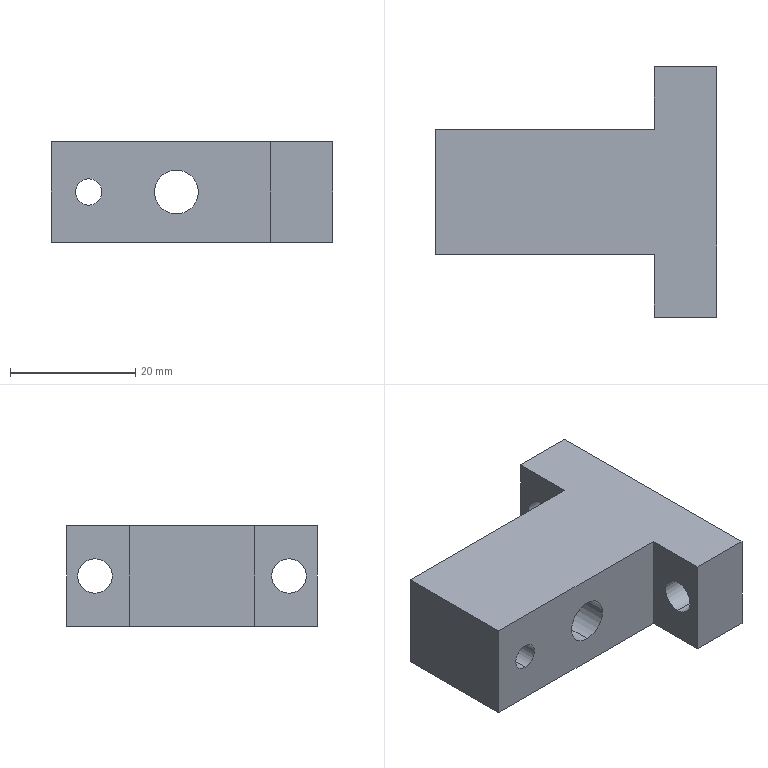Part | STEP file | 11-FG-E01311 | 1 solid | 24 faces | box 45 x 40 x 16 mm | volume 15803 mm3 | cylinder 12 | plane 12 | commonest cylinder face diameters 5 x4 5.5 x4 4.2 x2 7 x2
STEP:
#1=CARTESIAN_POINT('',(15.5,-5.5,10.5));
#2=VERTEX_POINT('',#1);
#3=CARTESIAN_POINT('',(15.5,-5.5,5.5));
#4=VERTEX_POINT('',#3);
#5=CARTESIAN_POINT('',(15.5,-5.5,8.));
#6=DIRECTION('',(1.,0.,0.));
#7=DIRECTION('',(0.,0.,-1.));
#8=AXIS2_PLACEMENT_3D('',#5,#6,#7);
#9=CIRCLE('',#8,2.5);
#10=EDGE_CURVE('',#2,#4,#9,.T.);
#11=ORIENTED_EDGE('',*,*,#10,.F.);
#12=CARTESIAN_POINT('',(22.5,-5.5,10.5));
#13=VERTEX_POINT('',#12);
#14=CARTESIAN_POINT('',(15.5,-5.5,10.5));
#15=DIRECTION('',(1.,0.,0.));
#16=VECTOR('',#15,1000.);
#17=LINE('',#14,#16);
#18=EDGE_CURVE('',#2,#13,#17,.T.);
#19=ORIENTED_EDGE('',*,*,#18,.T.);
#20=CARTESIAN_POINT('',(22.5,-5.5,5.5));
#21=VERTEX_POINT('',#20);
#22=CARTESIAN_POINT('',(22.5,-5.5,8.));
#23=DIRECTION('',(1.,0.,0.));
#24=DIRECTION('',(0.,0.,-1.));
#25=AXIS2_PLACEMENT_3D('',#22,#23,#24);
#26=CIRCLE('',#25,2.5);
#27=EDGE_CURVE('',#13,#21,#26,.T.);
#28=ORIENTED_EDGE('',*,*,#27,.T.);
#29=CARTESIAN_POINT('',(15.5,-5.5,5.5));
#30=DIRECTION('',(1.,0.,0.));
#31=VECTOR('',#30,1000.);
#32=LINE('',#29,#31);
#33=EDGE_CURVE('',#4,#21,#32,.T.);
#34=ORIENTED_EDGE('',*,*,#33,.F.);
#35=EDGE_LOOP('',(#11,#19,#28,#34));
#36=FACE_OUTER_BOUND('',#35,.T.);
#37=CARTESIAN_POINT('',(15.5,-5.5,8.));
#38=DIRECTION('',(1.,0.,0.));
#39=DIRECTION('',(0.,0.,-1.));
#40=AXIS2_PLACEMENT_3D('',#37,#38,#39);
#41=CYLINDRICAL_SURFACE('',#40,2.5);
#42=ADVANCED_FACE('',(#36),#41,.F.);
#43=CARTESIAN_POINT('',(15.5,5.5,10.5));
#44=VERTEX_POINT('',#43);
#45=CARTESIAN_POINT('',(15.5,5.5,5.5));
#46=VERTEX_POINT('',#45);
#47=CARTESIAN_POINT('',(15.5,5.5,8.));
#48=DIRECTION('',(1.,0.,0.));
#49=DIRECTION('',(0.,0.,-1.));
#50=AXIS2_PLACEMENT_3D('',#47,#48,#49);
#51=CIRCLE('',#50,2.5);
#52=EDGE_CURVE('',#44,#46,#51,.T.);
#53=ORIENTED_EDGE('',*,*,#52,.F.);
#54=CARTESIAN_POINT('',(22.5,5.5,10.5));
#55=VERTEX_POINT('',#54);
#56=CARTESIAN_POINT('',(15.5,5.5,10.5));
#57=DIRECTION('',(1.,0.,0.));
#58=VECTOR('',#57,1000.);
#59=LINE('',#56,#58);
#60=EDGE_CURVE('',#44,#55,#59,.T.);
#61=ORIENTED_EDGE('',*,*,#60,.T.);
#62=CARTESIAN_POINT('',(22.5,5.5,5.5));
#63=VERTEX_POINT('',#62);
#64=CARTESIAN_POINT('',(22.5,5.5,8.));
#65=DIRECTION('',(1.,0.,0.));
#66=DIRECTION('',(0.,0.,-1.));
#67=AXIS2_PLACEMENT_3D('',#64,#65,#66);
#68=CIRCLE('',#67,2.5);
#69=EDGE_CURVE('',#55,#63,#68,.T.);
#70=ORIENTED_EDGE('',*,*,#69,.T.);
#71=CARTESIAN_POINT('',(15.5,5.5,5.5));
#72=DIRECTION('',(1.,0.,0.));
#73=VECTOR('',#72,1000.);
#74=LINE('',#71,#73);
#75=EDGE_CURVE('',#46,#63,#74,.T.);
#76=ORIENTED_EDGE('',*,*,#75,.F.);
#77=EDGE_LOOP('',(#53,#61,#70,#76));
#78=FACE_OUTER_BOUND('',#77,.T.);
#79=CARTESIAN_POINT('',(15.5,5.5,8.));
#80=DIRECTION('',(1.,0.,0.));
#81=DIRECTION('',(0.,0.,-1.));
#82=AXIS2_PLACEMENT_3D('',#79,#80,#81);
#83=CYLINDRICAL_SURFACE('',#82,2.5);
#84=ADVANCED_FACE('',(#78),#83,.F.);
#85=CARTESIAN_POINT('',(22.5,-15.5,5.25));
#86=VERTEX_POINT('',#85);
#87=CARTESIAN_POINT('',(22.5,-15.5,10.75));
#88=VERTEX_POINT('',#87);
#89=CARTESIAN_POINT('',(22.5,-15.5,8.));
#90=DIRECTION('',(-1.,0.,0.));
#91=DIRECTION('',(0.,0.,1.));
#92=AXIS2_PLACEMENT_3D('',#89,#90,#91);
#93=CIRCLE('',#92,2.75);
#94=EDGE_CURVE('',#86,#88,#93,.T.);
#95=ORIENTED_EDGE('',*,*,#94,.F.);
#96=CARTESIAN_POINT('',(12.5,-15.5,5.25));
#97=VERTEX_POINT('',#96);
#98=CARTESIAN_POINT('',(27.5,-15.5,5.25));
#99=DIRECTION('',(-1.,0.,0.));
#100=VECTOR('',#99,1000.);
#101=LINE('',#98,#100);
#102=EDGE_CURVE('',#86,#97,#101,.T.);
#103=ORIENTED_EDGE('',*,*,#102,.T.);
#104=CARTESIAN_POINT('',(12.5,-15.5,10.75));
#105=VERTEX_POINT('',#104);
#106=CARTESIAN_POINT('',(12.5,-15.5,8.));
#107=DIRECTION('',(-1.,0.,0.));
#108=DIRECTION('',(0.,0.,1.));
#109=AXIS2_PLACEMENT_3D('',#106,#107,#108);
#110=CIRCLE('',#109,2.75);
#111=EDGE_CURVE('',#97,#105,#110,.T.);
#112=ORIENTED_EDGE('',*,*,#111,.T.);
#113=CARTESIAN_POINT('',(27.5,-15.5,10.75));
#114=DIRECTION('',(-1.,0.,0.));
#115=VECTOR('',#114,1000.);
#116=LINE('',#113,#115);
#117=EDGE_CURVE('',#88,#105,#116,.T.);
#118=ORIENTED_EDGE('',*,*,#117,.F.);
#119=EDGE_LOOP('',(#95,#103,#112,#118));
#120=FACE_OUTER_BOUND('',#119,.T.);
#121=CARTESIAN_POINT('',(27.5,-15.5,8.));
#122=DIRECTION('',(-1.,0.,0.));
#123=DIRECTION('',(0.,0.,1.));
#124=AXIS2_PLACEMENT_3D('',#121,#122,#123);
#125=CYLINDRICAL_SURFACE('',#124,2.75);
#126=ADVANCED_FACE('',(#120),#125,.F.);
#127=CARTESIAN_POINT('',(22.5,15.5,5.25));
#128=VERTEX_POINT('',#127);
#129=CARTESIAN_POINT('',(22.5,15.5,10.75));
#130=VERTEX_POINT('',#129);
#131=CARTESIAN_POINT('',(22.5,15.5,8.));
#132=DIRECTION('',(-1.,0.,0.));
#133=DIRECTION('',(0.,0.,1.));
#134=AXIS2_PLACEMENT_3D('',#131,#132,#133);
#135=CIRCLE('',#134,2.75);
#136=EDGE_CURVE('',#128,#130,#135,.T.);
#137=ORIENTED_EDGE('',*,*,#136,.F.);
#138=CARTESIAN_POINT('',(12.5,15.5,5.25));
#139=VERTEX_POINT('',#138);
#140=CARTESIAN_POINT('',(27.5,15.5,5.25));
#141=DIRECTION('',(-1.,0.,0.));
#142=VECTOR('',#141,1000.);
#143=LINE('',#140,#142);
#144=EDGE_CURVE('',#128,#139,#143,.T.);
#145=ORIENTED_EDGE('',*,*,#144,.T.);
#146=CARTESIAN_POINT('',(12.5,15.5,10.75));
#147=VERTEX_POINT('',#146);
#148=CARTESIAN_POINT('',(12.5,15.5,8.));
#149=DIRECTION('',(-1.,0.,0.));
#150=DIRECTION('',(0.,0.,1.));
#151=AXIS2_PLACEMENT_3D('',#148,#149,#150);
#152=CIRCLE('',#151,2.75);
#153=EDGE_CURVE('',#139,#147,#152,.T.);
#154=ORIENTED_EDGE('',*,*,#153,.T.);
#155=CARTESIAN_POINT('',(27.5,15.5,10.75));
#156=DIRECTION('',(-1.,0.,0.));
#157=VECTOR('',#156,1000.);
#158=LINE('',#155,#157);
#159=EDGE_CURVE('',#130,#147,#158,.T.);
#160=ORIENTED_EDGE('',*,*,#159,.F.);
#161=EDGE_LOOP('',(#137,#145,#154,#160));
#162=FACE_OUTER_BOUND('',#161,.T.);
#163=CARTESIAN_POINT('',(27.5,15.5,8.));
#164=DIRECTION('',(-1.,0.,0.));
#165=DIRECTION('',(0.,0.,1.));
#166=AXIS2_PLACEMENT_3D('',#163,#164,#165);
#167=CYLINDRICAL_SURFACE('',#166,2.75);
#168=ADVANCED_FACE('',(#162),#167,.F.);
#169=CARTESIAN_POINT('',(-16.5,10.,10.1));
#170=VERTEX_POINT('',#169);
#171=CARTESIAN_POINT('',(-16.5,10.,5.9));
#172=VERTEX_POINT('',#171);
#173=CARTESIAN_POINT('',(-16.5,10.,8.));
#174=DIRECTION('',(0.,-1.,0.));
#175=DIRECTION('',(0.,0.,-1.));
#176=AXIS2_PLACEMENT_3D('',#173,#174,#175);
#177=CIRCLE('',#176,2.1);
#178=EDGE_CURVE('',#170,#172,#177,.T.);
#179=ORIENTED_EDGE('',*,*,#178,.F.);
#180=CARTESIAN_POINT('',(-16.5,-10.,10.1));
#181=VERTEX_POINT('',#180);
#182=CARTESIAN_POINT('',(-16.5,-10.,10.1));
#183=DIRECTION('',(0.,-1.,0.));
#184=VECTOR('',#183,1000.);
#185=LINE('',#182,#184);
#186=EDGE_CURVE('',#170,#181,#185,.T.);
#187=ORIENTED_EDGE('',*,*,#186,.T.);
#188=CARTESIAN_POINT('',(-16.5,-10.,5.9));
#189=VERTEX_POINT('',#188);
#190=CARTESIAN_POINT('',(-16.5,-10.,8.));
#191=DIRECTION('',(0.,-1.,0.));
#192=DIRECTION('',(0.,0.,-1.));
#193=AXIS2_PLACEMENT_3D('',#190,#191,#192);
#194=CIRCLE('',#193,2.1);
#195=EDGE_CURVE('',#181,#189,#194,.T.);
#196=ORIENTED_EDGE('',*,*,#195,.T.);
#197=CARTESIAN_POINT('',(-16.5,-10.,5.9));
#198=DIRECTION('',(0.,-1.,0.));
#199=VECTOR('',#198,1000.);
#200=LINE('',#197,#199);
#201=EDGE_CURVE('',#172,#189,#200,.T.);
#202=ORIENTED_EDGE('',*,*,#201,.F.);
#203=EDGE_LOOP('',(#179,#187,#196,#202));
#204=FACE_OUTER_BOUND('',#203,.T.);
#205=CARTESIAN_POINT('',(-16.5,-10.,8.));
#206=DIRECTION('',(0.,-1.,0.));
#207=DIRECTION('',(0.,0.,-1.));
#208=AXIS2_PLACEMENT_3D('',#205,#206,#207);
#209=CYLINDRICAL_SURFACE('',#208,2.1);
#210=ADVANCED_FACE('',(#204),#209,.F.);
#211=CARTESIAN_POINT('',(-2.5,10.,11.5));
#212=VERTEX_POINT('',#211);
#213=CARTESIAN_POINT('',(-2.5,10.,4.5));
#214=VERTEX_POINT('',#213);
#215=CARTESIAN_POINT('',(-2.5,10.,8.));
#216=DIRECTION('',(0.,-1.,0.));
#217=DIRECTION('',(0.,0.,-1.));
#218=AXIS2_PLACEMENT_3D('',#215,#216,#217);
#219=CIRCLE('',#218,3.5);
#220=EDGE_CURVE('',#212,#214,#219,.T.);
#221=ORIENTED_EDGE('',*,*,#220,.F.);
#222=CARTESIAN_POINT('',(-2.5,-10.,11.5));
#223=VERTEX_POINT('',#222);
#224=CARTESIAN_POINT('',(-2.5,-10.,11.5));
#225=DIRECTION('',(0.,-1.,0.));
#226=VECTOR('',#225,1000.);
#227=LINE('',#224,#226);
#228=EDGE_CURVE('',#212,#223,#227,.T.);
#229=ORIENTED_EDGE('',*,*,#228,.T.);
#230=CARTESIAN_POINT('',(-2.5,-10.,4.5));
#231=VERTEX_POINT('',#230);
#232=CARTESIAN_POINT('',(-2.5,-10.,8.));
#233=DIRECTION('',(0.,-1.,0.));
#234=DIRECTION('',(0.,0.,-1.));
#235=AXIS2_PLACEMENT_3D('',#232,#233,#234);
#236=CIRCLE('',#235,3.5);
#237=EDGE_CURVE('',#223,#231,#236,.T.);
#238=ORIENTED_EDGE('',*,*,#237,.T.);
#239=CARTESIAN_POINT('',(-2.5,-10.,4.5));
#240=DIRECTION('',(0.,-1.,0.));
#241=VECTOR('',#240,1000.);
#242=LINE('',#239,#241);
#243=EDGE_CURVE('',#214,#231,#242,.T.);
#244=ORIENTED_EDGE('',*,*,#243,.F.);
#245=EDGE_LOOP('',(#221,#229,#238,#244));
#246=FACE_OUTER_BOUND('',#245,.T.);
#247=CARTESIAN_POINT('',(-2.5,-10.,8.));
#248=DIRECTION('',(0.,-1.,0.));
#249=DIRECTION('',(0.,0.,-1.));
#250=AXIS2_PLACEMENT_3D('',#247,#248,#249);
#251=CYLINDRICAL_SURFACE('',#250,3.5);
#252=ADVANCED_FACE('',(#246),#251,.F.);
#253=CARTESIAN_POINT('',(22.5,-5.5,8.));
#254=DIRECTION('',(1.,0.,0.));
#255=DIRECTION('',(0.,0.,-1.));
#256=AXIS2_PLACEMENT_3D('',#253,#254,#255);
#257=CIRCLE('',#256,2.5);
#258=EDGE_CURVE('',#21,#13,#257,.T.);
#259=ORIENTED_EDGE('',*,*,#258,.F.);
#260=ORIENTED_EDGE('',*,*,#27,.F.);
#261=EDGE_LOOP('',(#259,#260));
#262=FACE_BOUND('',#261,.T.);
#263=CARTESIAN_POINT('',(22.5,5.5,8.));
#264=DIRECTION('',(1.,0.,0.));
#265=DIRECTION('',(0.,0.,-1.));
#266=AXIS2_PLACEMENT_3D('',#263,#264,#265);
#267=CIRCLE('',#266,2.5);
#268=EDGE_CURVE('',#63,#55,#267,.T.);
#269=ORIENTED_EDGE('',*,*,#268,.F.);
#270=ORIENTED_EDGE('',*,*,#69,.F.);
#271=EDGE_LOOP('',(#269,#270));
#272=FACE_BOUND('',#271,.T.);
#273=CARTESIAN_POINT('',(22.5,-15.5,8.));
#274=DIRECTION('',(-1.,0.,0.));
#275=DIRECTION('',(0.,0.,1.));
#276=AXIS2_PLACEMENT_3D('',#273,#274,#275);
#277=CIRCLE('',#276,2.75);
#278=EDGE_CURVE('',#88,#86,#277,.T.);
#279=ORIENTED_EDGE('',*,*,#278,.T.);
#280=ORIENTED_EDGE('',*,*,#94,.T.);
#281=EDGE_LOOP('',(#279,#280));
#282=FACE_BOUND('',#281,.T.);
#283=CARTESIAN_POINT('',(22.5,15.5,8.));
#284=DIRECTION('',(-1.,0.,0.));
#285=DIRECTION('',(0.,0.,1.));
#286=AXIS2_PLACEMENT_3D('',#283,#284,#285);
#287=CIRCLE('',#286,2.75);
#288=EDGE_CURVE('',#130,#128,#287,.T.);
#289=ORIENTED_EDGE('',*,*,#288,.T.);
#290=ORIENTED_EDGE('',*,*,#136,.T.);
#291=EDGE_LOOP('',(#289,#290));
#292=FACE_BOUND('',#291,.T.);
#293=CARTESIAN_POINT('',(22.5,-20.,0.));
#294=VERTEX_POINT('',#293);
#295=CARTESIAN_POINT('',(22.5,20.,0.));
#296=VERTEX_POINT('',#295);
#297=CARTESIAN_POINT('',(22.5,10.,0.));
#298=DIRECTION('',(0.,1.,0.));
#299=VECTOR('',#298,1000.);
#300=LINE('',#297,#299);
#301=EDGE_CURVE('',#294,#296,#300,.T.);
#302=ORIENTED_EDGE('',*,*,#301,.T.);
#303=CARTESIAN_POINT('',(22.5,20.,16.));
#304=VERTEX_POINT('',#303);
#305=CARTESIAN_POINT('',(22.5,20.,16.));
#306=DIRECTION('',(0.,0.,1.));
#307=VECTOR('',#306,1000.);
#308=LINE('',#305,#307);
#309=EDGE_CURVE('',#296,#304,#308,.T.);
#310=ORIENTED_EDGE('',*,*,#309,.T.);
#311=CARTESIAN_POINT('',(22.5,-20.,16.));
#312=VERTEX_POINT('',#311);
#313=CARTESIAN_POINT('',(22.5,55.706,16.));
#314=DIRECTION('',(0.,-1.,0.));
#315=VECTOR('',#314,1000.);
#316=LINE('',#313,#315);
#317=EDGE_CURVE('',#304,#312,#316,.T.);
#318=ORIENTED_EDGE('',*,*,#317,.T.);
#319=CARTESIAN_POINT('',(22.5,-20.,16.));
#320=DIRECTION('',(0.,0.,-1.));
#321=VECTOR('',#320,1000.);
#322=LINE('',#319,#321);
#323=EDGE_CURVE('',#312,#294,#322,.T.);
#324=ORIENTED_EDGE('',*,*,#323,.T.);
#325=EDGE_LOOP('',(#302,#310,#318,#324));
#326=FACE_OUTER_BOUND('',#325,.T.);
#327=CARTESIAN_POINT('',(22.5,10.,8.));
#328=DIRECTION('',(-1.,0.,0.));
#329=DIRECTION('',(0.,0.,1.));
#330=AXIS2_PLACEMENT_3D('',#327,#328,#329);
#331=PLANE('',#330);
#332=ADVANCED_FACE('',(#262,#272,#282,#292,#326),#331,.F.);
#333=CARTESIAN_POINT('',(-16.5,10.,8.));
#334=DIRECTION('',(0.,-1.,0.));
#335=DIRECTION('',(0.,0.,-1.));
#336=AXIS2_PLACEMENT_3D('',#333,#334,#335);
#337=CIRCLE('',#336,2.1);
#338=EDGE_CURVE('',#172,#170,#337,.T.);
#339=ORIENTED_EDGE('',*,*,#338,.T.);
#340=ORIENTED_EDGE('',*,*,#178,.T.);
#341=EDGE_LOOP('',(#339,#340));
#342=FACE_BOUND('',#341,.T.);
#343=CARTESIAN_POINT('',(-2.5,10.,8.));
#344=DIRECTION('',(0.,-1.,0.));
#345=DIRECTION('',(0.,0.,-1.));
#346=AXIS2_PLACEMENT_3D('',#343,#344,#345);
#347=CIRCLE('',#346,3.5);
#348=EDGE_CURVE('',#214,#212,#347,.T.);
#349=ORIENTED_EDGE('',*,*,#348,.T.);
#350=ORIENTED_EDGE('',*,*,#220,.T.);
#351=EDGE_LOOP('',(#349,#350));
#352=FACE_BOUND('',#351,.T.);
#353=CARTESIAN_POINT('',(-22.5,10.,16.));
#354=VERTEX_POINT('',#353);
#355=CARTESIAN_POINT('',(12.5,10.,16.));
#356=VERTEX_POINT('',#355);
#357=CARTESIAN_POINT('',(-22.5,10.,16.));
#358=DIRECTION('',(1.,0.,0.));
#359=VECTOR('',#358,1000.);
#360=LINE('',#357,#359);
#361=EDGE_CURVE('',#354,#356,#360,.T.);
#362=ORIENTED_EDGE('',*,*,#361,.T.);
#363=CARTESIAN_POINT('',(12.5,10.,0.));
#364=VERTEX_POINT('',#363);
#365=CARTESIAN_POINT('',(12.5,10.,16.));
#366=DIRECTION('',(0.,0.,-1.));
#367=VECTOR('',#366,1000.);
#368=LINE('',#365,#367);
#369=EDGE_CURVE('',#356,#364,#368,.T.);
#370=ORIENTED_EDGE('',*,*,#369,.T.);
#371=CARTESIAN_POINT('',(-22.5,10.,0.));
#372=VERTEX_POINT('',#371);
#373=CARTESIAN_POINT('',(-22.5,10.,0.));
#374=DIRECTION('',(-1.,0.,0.));
#375=VECTOR('',#374,1000.);
#376=LINE('',#373,#375);
#377=EDGE_CURVE('',#364,#372,#376,.T.);
#378=ORIENTED_EDGE('',*,*,#377,.T.);
#379=CARTESIAN_POINT('',(-22.5,10.,8.));
#380=DIRECTION('',(0.,0.,-1.));
#381=VECTOR('',#380,1000.);
#382=LINE('',#379,#381);
#383=EDGE_CURVE('',#354,#372,#382,.T.);
#384=ORIENTED_EDGE('',*,*,#383,.F.);
#385=EDGE_LOOP('',(#362,#370,#378,#384));
#386=FACE_OUTER_BOUND('',#385,.T.);
#387=CARTESIAN_POINT('',(-22.5,10.,8.));
#388=DIRECTION('',(0.,-1.,0.));
#389=DIRECTION('',(0.,0.,-1.));
#390=AXIS2_PLACEMENT_3D('',#387,#388,#389);
#391=PLANE('',#390);
#392=ADVANCED_FACE('',(#342,#352,#386),#391,.F.);
#393=CARTESIAN_POINT('',(-22.5,-10.,0.));
#394=VERTEX_POINT('',#393);
#395=CARTESIAN_POINT('',(-22.5,10.,0.));
#396=DIRECTION('',(0.,-1.,0.));
#397=VECTOR('',#396,1000.);
#398=LINE('',#395,#397);
#399=EDGE_CURVE('',#372,#394,#398,.T.);
#400=ORIENTED_EDGE('',*,*,#399,.T.);
#401=CARTESIAN_POINT('',(-22.5,-10.,16.));
#402=VERTEX_POINT('',#401);
#403=CARTESIAN_POINT('',(-22.5,-10.,8.));
#404=DIRECTION('',(0.,0.,-1.));
#405=VECTOR('',#404,1000.);
#406=LINE('',#403,#405);
#407=EDGE_CURVE('',#402,#394,#406,.T.);
#408=ORIENTED_EDGE('',*,*,#407,.F.);
#409=CARTESIAN_POINT('',(-22.5,55.706,16.));
#410=DIRECTION('',(0.,-1.,0.));
#411=VECTOR('',#410,1000.);
#412=LINE('',#409,#411);
#413=EDGE_CURVE('',#354,#402,#412,.T.);
#414=ORIENTED_EDGE('',*,*,#413,.F.);
#415=ORIENTED_EDGE('',*,*,#383,.T.);
#416=EDGE_LOOP('',(#400,#408,#414,#415));
#417=FACE_OUTER_BOUND('',#416,.T.);
#418=CARTESIAN_POINT('',(-22.5,10.,8.));
#419=DIRECTION('',(1.,0.,0.));
#420=DIRECTION('',(0.,1.,0.));
#421=AXIS2_PLACEMENT_3D('',#418,#419,#420);
#422=PLANE('',#421);
#423=ADVANCED_FACE('',(#417),#422,.F.);
#424=CARTESIAN_POINT('',(-16.5,-10.,8.));
#425=DIRECTION('',(0.,-1.,0.));
#426=DIRECTION('',(0.,0.,-1.));
#427=AXIS2_PLACEMENT_3D('',#424,#425,#426);
#428=CIRCLE('',#427,2.1);
#429=EDGE_CURVE('',#189,#181,#428,.T.);
#430=ORIENTED_EDGE('',*,*,#429,.F.);
#431=ORIENTED_EDGE('',*,*,#195,.F.);
#432=EDGE_LOOP('',(#430,#431));
#433=FACE_BOUND('',#432,.T.);
#434=CARTESIAN_POINT('',(-2.5,-10.,8.));
#435=DIRECTION('',(0.,-1.,0.));
#436=DIRECTION('',(0.,0.,-1.));
#437=AXIS2_PLACEMENT_3D('',#434,#435,#436);
#438=CIRCLE('',#437,3.5);
#439=EDGE_CURVE('',#231,#223,#438,.T.);
#440=ORIENTED_EDGE('',*,*,#439,.F.);
#441=ORIENTED_EDGE('',*,*,#237,.F.);
#442=EDGE_LOOP('',(#440,#441));
#443=FACE_BOUND('',#442,.T.);
#444=CARTESIAN_POINT('',(12.5,-10.,0.));
#445=VERTEX_POINT('',#444);
#446=CARTESIAN_POINT('',(-22.5,-10.,0.));
#447=DIRECTION('',(1.,0.,0.));
#448=VECTOR('',#447,1000.);
#449=LINE('',#446,#448);
#450=EDGE_CURVE('',#394,#445,#449,.T.);
#451=ORIENTED_EDGE('',*,*,#450,.T.);
#452=CARTESIAN_POINT('',(12.5,-10.,16.));
#453=VERTEX_POINT('',#452);
#454=CARTESIAN_POINT('',(12.5,-10.,16.));
#455=DIRECTION('',(0.,0.,1.));
#456=VECTOR('',#455,1000.);
#457=LINE('',#454,#456);
#458=EDGE_CURVE('',#445,#453,#457,.T.);
#459=ORIENTED_EDGE('',*,*,#458,.T.);
#460=CARTESIAN_POINT('',(-22.5,-10.,16.));
#461=DIRECTION('',(-1.,0.,0.));
#462=VECTOR('',#461,1000.);
#463=LINE('',#460,#462);
#464=EDGE_CURVE('',#453,#402,#463,.T.);
#465=ORIENTED_EDGE('',*,*,#464,.T.);
#466=ORIENTED_EDGE('',*,*,#407,.T.);
#467=EDGE_LOOP('',(#451,#459,#465,#466));
#468=FACE_OUTER_BOUND('',#467,.T.);
#469=CARTESIAN_POINT('',(-22.5,-10.,8.));
#470=DIRECTION('',(0.,1.,0.));
#471=DIRECTION('',(0.,0.,1.));
#472=AXIS2_PLACEMENT_3D('',#469,#470,#471);
#473=PLANE('',#472);
#474=ADVANCED_FACE('',(#433,#443,#468),#473,.F.);
#475=ORIENTED_EDGE('',*,*,#301,.F.);
#476=CARTESIAN_POINT('',(12.5,-20.,0.));
#477=VERTEX_POINT('',#476);
#478=CARTESIAN_POINT('',(12.5,-20.,0.));
#479=DIRECTION('',(1.,0.,0.));
#480=VECTOR('',#479,1000.);
#481=LINE('',#478,#480);
#482=EDGE_CURVE('',#477,#294,#481,.T.);
#483=ORIENTED_EDGE('',*,*,#482,.F.);
#484=CARTESIAN_POINT('',(12.5,-10.,0.));
#485=DIRECTION('',(0.,1.,0.));
#486=VECTOR('',#485,1000.);
#487=LINE('',#484,#486);
#488=EDGE_CURVE('',#477,#445,#487,.T.);
#489=ORIENTED_EDGE('',*,*,#488,.T.);
#490=ORIENTED_EDGE('',*,*,#450,.F.);
#491=ORIENTED_EDGE('',*,*,#399,.F.);
#492=ORIENTED_EDGE('',*,*,#377,.F.);
#493=CARTESIAN_POINT('',(12.5,20.,0.));
#494=VERTEX_POINT('',#493);
#495=CARTESIAN_POINT('',(12.5,10.,0.));
#496=DIRECTION('',(0.,1.,0.));
#497=VECTOR('',#496,1000.);
#498=LINE('',#495,#497);
#499=EDGE_CURVE('',#364,#494,#498,.T.);
#500=ORIENTED_EDGE('',*,*,#499,.T.);
#501=CARTESIAN_POINT('',(12.5,20.,0.));
#502=DIRECTION('',(1.,0.,0.));
#503=VECTOR('',#502,1000.);
#504=LINE('',#501,#503);
#505=EDGE_CURVE('',#494,#296,#504,.T.);
#506=ORIENTED_EDGE('',*,*,#505,.T.);
#507=EDGE_LOOP('',(#475,#483,#489,#490,#491,#492,#500,#506));
#508=FACE_OUTER_BOUND('',#507,.T.);
#509=CARTESIAN_POINT('',(22.5,-10.,0.));
#510=DIRECTION('',(0.,0.,1.));
#511=DIRECTION('',(1.,0.,0.));
#512=AXIS2_PLACEMENT_3D('',#509,#510,#511);
#513=PLANE('',#512);
#514=ADVANCED_FACE('',(#508),#513,.F.);
#515=ORIENTED_EDGE('',*,*,#361,.F.);
#516=ORIENTED_EDGE('',*,*,#413,.T.);
#517=ORIENTED_EDGE('',*,*,#464,.F.);
#518=CARTESIAN_POINT('',(12.5,-20.,16.));
#519=VERTEX_POINT('',#518);
#520=CARTESIAN_POINT('',(12.5,-10.,16.));
#521=DIRECTION('',(0.,-1.,0.));
#522=VECTOR('',#521,1000.);
#523=LINE('',#520,#522);
#524=EDGE_CURVE('',#453,#519,#523,.T.);
#525=ORIENTED_EDGE('',*,*,#524,.T.);
#526=CARTESIAN_POINT('',(12.5,-20.,16.));
#527=DIRECTION('',(1.,0.,0.));
#528=VECTOR('',#527,1000.);
#529=LINE('',#526,#528);
#530=EDGE_CURVE('',#519,#312,#529,.T.);
#531=ORIENTED_EDGE('',*,*,#530,.T.);
#532=ORIENTED_EDGE('',*,*,#317,.F.);
#533=CARTESIAN_POINT('',(12.5,20.,16.));
#534=VERTEX_POINT('',#533);
#535=CARTESIAN_POINT('',(12.5,20.,16.));
#536=DIRECTION('',(1.,0.,0.));
#537=VECTOR('',#536,1000.);
#538=LINE('',#535,#537);
#539=EDGE_CURVE('',#534,#304,#538,.T.);
#540=ORIENTED_EDGE('',*,*,#539,.F.);
#541=CARTESIAN_POINT('',(12.5,10.,16.));
#542=DIRECTION('',(0.,-1.,0.));
#543=VECTOR('',#542,1000.);
#544=LINE('',#541,#543);
#545=EDGE_CURVE('',#534,#356,#544,.T.);
#546=ORIENTED_EDGE('',*,*,#545,.T.);
#547=EDGE_LOOP('',(#515,#516,#517,#525,#531,#532,#540,#546));
#548=FACE_OUTER_BOUND('',#547,.T.);
#549=CARTESIAN_POINT('',(-22.5,55.706,16.));
#550=DIRECTION('',(0.,0.,1.));
#551=DIRECTION('',(1.,0.,0.));
#552=AXIS2_PLACEMENT_3D('',#549,#550,#551);
#553=PLANE('',#552);
#554=ADVANCED_FACE('',(#548),#553,.T.);
#555=ORIENTED_EDGE('',*,*,#228,.F.);
#556=ORIENTED_EDGE('',*,*,#348,.F.);
#557=ORIENTED_EDGE('',*,*,#243,.T.);
#558=ORIENTED_EDGE('',*,*,#439,.T.);
#559=EDGE_LOOP('',(#555,#556,#557,#558));
#560=FACE_OUTER_BOUND('',#559,.T.);
#561=CARTESIAN_POINT('',(-2.5,-10.,8.));
#562=DIRECTION('',(0.,-1.,0.));
#563=DIRECTION('',(0.,0.,-1.));
#564=AXIS2_PLACEMENT_3D('',#561,#562,#563);
#565=CYLINDRICAL_SURFACE('',#564,3.5);
#566=ADVANCED_FACE('',(#560),#565,.F.);
#567=ORIENTED_EDGE('',*,*,#186,.F.);
#568=ORIENTED_EDGE('',*,*,#338,.F.);
#569=ORIENTED_EDGE('',*,*,#201,.T.);
#570=ORIENTED_EDGE('',*,*,#429,.T.);
#571=EDGE_LOOP('',(#567,#568,#569,#570));
#572=FACE_OUTER_BOUND('',#571,.T.);
#573=CARTESIAN_POINT('',(-16.5,-10.,8.));
#574=DIRECTION('',(0.,-1.,0.));
#575=DIRECTION('',(0.,0.,-1.));
#576=AXIS2_PLACEMENT_3D('',#573,#574,#575);
#577=CYLINDRICAL_SURFACE('',#576,2.1);
#578=ADVANCED_FACE('',(#572),#577,.F.);
#579=ORIENTED_EDGE('',*,*,#309,.F.);
#580=ORIENTED_EDGE('',*,*,#505,.F.);
#581=CARTESIAN_POINT('',(12.5,20.,16.));
#582=DIRECTION('',(0.,0.,1.));
#583=VECTOR('',#582,1000.);
#584=LINE('',#581,#583);
#585=EDGE_CURVE('',#494,#534,#584,.T.);
#586=ORIENTED_EDGE('',*,*,#585,.T.);
#587=ORIENTED_EDGE('',*,*,#539,.T.);
#588=EDGE_LOOP('',(#579,#580,#586,#587));
#589=FACE_OUTER_BOUND('',#588,.T.);
#590=CARTESIAN_POINT('',(12.5,20.,16.));
#591=DIRECTION('',(0.,1.,0.));
#592=DIRECTION('',(0.,0.,1.));
#593=AXIS2_PLACEMENT_3D('',#590,#591,#592);
#594=PLANE('',#593);
#595=ADVANCED_FACE('',(#589),#594,.T.);
#596=CARTESIAN_POINT('',(12.5,15.5,8.));
#597=DIRECTION('',(-1.,0.,0.));
#598=DIRECTION('',(0.,0.,1.));
#599=AXIS2_PLACEMENT_3D('',#596,#597,#598);
#600=CIRCLE('',#599,2.75);
#601=EDGE_CURVE('',#147,#139,#600,.T.);
#602=ORIENTED_EDGE('',*,*,#601,.F.);
#603=ORIENTED_EDGE('',*,*,#153,.F.);
#604=EDGE_LOOP('',(#602,#603));
#605=FACE_BOUND('',#604,.T.);
#606=ORIENTED_EDGE('',*,*,#545,.F.);
#607=ORIENTED_EDGE('',*,*,#585,.F.);
#608=ORIENTED_EDGE('',*,*,#499,.F.);
#609=ORIENTED_EDGE('',*,*,#369,.F.);
#610=EDGE_LOOP('',(#606,#607,#608,#609));
#611=FACE_OUTER_BOUND('',#610,.T.);
#612=CARTESIAN_POINT('',(12.5,0.,0.));
#613=DIRECTION('',(-1.,0.,0.));
#614=DIRECTION('',(0.,0.,1.));
#615=AXIS2_PLACEMENT_3D('',#612,#613,#614);
#616=PLANE('',#615);
#617=ADVANCED_FACE('',(#605,#611),#616,.T.);
#618=ORIENTED_EDGE('',*,*,#323,.F.);
#619=ORIENTED_EDGE('',*,*,#530,.F.);
#620=CARTESIAN_POINT('',(12.5,-20.,16.));
#621=DIRECTION('',(0.,0.,-1.));
#622=VECTOR('',#621,1000.);
#623=LINE('',#620,#622);
#624=EDGE_CURVE('',#519,#477,#623,.T.);
#625=ORIENTED_EDGE('',*,*,#624,.T.);
#626=ORIENTED_EDGE('',*,*,#482,.T.);
#627=EDGE_LOOP('',(#618,#619,#625,#626));
#628=FACE_OUTER_BOUND('',#627,.T.);
#629=CARTESIAN_POINT('',(12.5,-20.,16.));
#630=DIRECTION('',(0.,-1.,0.));
#631=DIRECTION('',(0.,0.,-1.));
#632=AXIS2_PLACEMENT_3D('',#629,#630,#631);
#633=PLANE('',#632);
#634=ADVANCED_FACE('',(#628),#633,.T.);
#635=CARTESIAN_POINT('',(12.5,-15.5,8.));
#636=DIRECTION('',(-1.,0.,0.));
#637=DIRECTION('',(0.,0.,1.));
#638=AXIS2_PLACEMENT_3D('',#635,#636,#637);
#639=CIRCLE('',#638,2.75);
#640=EDGE_CURVE('',#105,#97,#639,.T.);
#641=ORIENTED_EDGE('',*,*,#640,.F.);
#642=ORIENTED_EDGE('',*,*,#111,.F.);
#643=EDGE_LOOP('',(#641,#642));
#644=FACE_BOUND('',#643,.T.);
#645=ORIENTED_EDGE('',*,*,#458,.F.);
#646=ORIENTED_EDGE('',*,*,#488,.F.);
#647=ORIENTED_EDGE('',*,*,#624,.F.);
#648=ORIENTED_EDGE('',*,*,#524,.F.);
#649=EDGE_LOOP('',(#645,#646,#647,#648));
#650=FACE_OUTER_BOUND('',#649,.T.);
#651=CARTESIAN_POINT('',(12.5,0.,0.));
#652=DIRECTION('',(-1.,0.,0.));
#653=DIRECTION('',(0.,0.,1.));
#654=AXIS2_PLACEMENT_3D('',#651,#652,#653);
#655=PLANE('',#654);
#656=ADVANCED_FACE('',(#644,#650),#655,.T.);
#657=ORIENTED_EDGE('',*,*,#144,.F.);
#658=ORIENTED_EDGE('',*,*,#288,.F.);
#659=ORIENTED_EDGE('',*,*,#159,.T.);
#660=ORIENTED_EDGE('',*,*,#601,.T.);
#661=EDGE_LOOP('',(#657,#658,#659,#660));
#662=FACE_OUTER_BOUND('',#661,.T.);
#663=CARTESIAN_POINT('',(27.5,15.5,8.));
#664=DIRECTION('',(-1.,0.,0.));
#665=DIRECTION('',(0.,0.,1.));
#666=AXIS2_PLACEMENT_3D('',#663,#664,#665);
#667=CYLINDRICAL_SURFACE('',#666,2.75);
#668=ADVANCED_FACE('',(#662),#667,.F.);
#669=ORIENTED_EDGE('',*,*,#102,.F.);
#670=ORIENTED_EDGE('',*,*,#278,.F.);
#671=ORIENTED_EDGE('',*,*,#117,.T.);
#672=ORIENTED_EDGE('',*,*,#640,.T.);
#673=EDGE_LOOP('',(#669,#670,#671,#672));
#674=FACE_OUTER_BOUND('',#673,.T.);
#675=CARTESIAN_POINT('',(27.5,-15.5,8.));
#676=DIRECTION('',(-1.,0.,0.));
#677=DIRECTION('',(0.,0.,1.));
#678=AXIS2_PLACEMENT_3D('',#675,#676,#677);
#679=CYLINDRICAL_SURFACE('',#678,2.75);
#680=ADVANCED_FACE('',(#674),#679,.F.);
#681=ORIENTED_EDGE('',*,*,#60,.F.);
#682=CARTESIAN_POINT('',(15.5,5.5,8.));
#683=DIRECTION('',(1.,0.,0.));
#684=DIRECTION('',(0.,0.,-1.));
#685=AXIS2_PLACEMENT_3D('',#682,#683,#684);
#686=CIRCLE('',#685,2.5);
#687=EDGE_CURVE('',#46,#44,#686,.T.);
#688=ORIENTED_EDGE('',*,*,#687,.F.);
#689=ORIENTED_EDGE('',*,*,#75,.T.);
#690=ORIENTED_EDGE('',*,*,#268,.T.);
#691=EDGE_LOOP('',(#681,#688,#689,#690));
#692=FACE_OUTER_BOUND('',#691,.T.);
#693=CARTESIAN_POINT('',(15.5,5.5,8.));
#694=DIRECTION('',(1.,0.,0.));
#695=DIRECTION('',(0.,0.,-1.));
#696=AXIS2_PLACEMENT_3D('',#693,#694,#695);
#697=CYLINDRICAL_SURFACE('',#696,2.5);
#698=ADVANCED_FACE('',(#692),#697,.F.);
#699=ORIENTED_EDGE('',*,*,#687,.T.);
#700=ORIENTED_EDGE('',*,*,#52,.T.);
#701=EDGE_LOOP('',(#699,#700));
#702=FACE_OUTER_BOUND('',#701,.T.);
#703=CARTESIAN_POINT('',(15.5,5.5,8.));
#704=DIRECTION('',(1.,0.,0.));
#705=DIRECTION('',(0.,0.,-1.));
#706=AXIS2_PLACEMENT_3D('',#703,#704,#705);
#707=PLANE('',#706);
#708=ADVANCED_FACE('',(#702),#707,.T.);
#709=ORIENTED_EDGE('',*,*,#18,.F.);
#710=CARTESIAN_POINT('',(15.5,-5.5,8.));
#711=DIRECTION('',(1.,0.,0.));
#712=DIRECTION('',(0.,0.,-1.));
#713=AXIS2_PLACEMENT_3D('',#710,#711,#712);
#714=CIRCLE('',#713,2.5);
#715=EDGE_CURVE('',#4,#2,#714,.T.);
#716=ORIENTED_EDGE('',*,*,#715,.F.);
#717=ORIENTED_EDGE('',*,*,#33,.T.);
#718=ORIENTED_EDGE('',*,*,#258,.T.);
#719=EDGE_LOOP('',(#709,#716,#717,#718));
#720=FACE_OUTER_BOUND('',#719,.T.);
#721=CARTESIAN_POINT('',(15.5,-5.5,8.));
#722=DIRECTION('',(1.,0.,0.));
#723=DIRECTION('',(0.,0.,-1.));
#724=AXIS2_PLACEMENT_3D('',#721,#722,#723);
#725=CYLINDRICAL_SURFACE('',#724,2.5);
#726=ADVANCED_FACE('',(#720),#725,.F.);
#727=ORIENTED_EDGE('',*,*,#715,.T.);
#728=ORIENTED_EDGE('',*,*,#10,.T.);
#729=EDGE_LOOP('',(#727,#728));
#730=FACE_OUTER_BOUND('',#729,.T.);
#731=CARTESIAN_POINT('',(15.5,-5.5,8.));
#732=DIRECTION('',(1.,0.,0.));
#733=DIRECTION('',(0.,0.,-1.));
#734=AXIS2_PLACEMENT_3D('',#731,#732,#733);
#735=PLANE('',#734);
#736=ADVANCED_FACE('',(#730),#735,.T.);
#737=CLOSED_SHELL('',(#42,#84,#126,#168,#210,#252,#332,#392,#423,#474,#514,#554,#566,#578,#595,#617,#634,#656,#668,#680,#698,#708,#726,#736));
#738=MANIFOLD_SOLID_BREP('',#737);
#739=CARTESIAN_POINT('',(0.,0.,0.));
#740=DIRECTION('',(0.,0.,1.));
#741=DIRECTION('',(1.,0.,0.));
#742=AXIS2_PLACEMENT_3D('',#739,#740,#741);
#743=(LENGTH_UNIT()NAMED_UNIT(*)SI_UNIT(.MILLI.,.METRE.));
#744=UNCERTAINTY_MEASURE_WITH_UNIT(LENGTH_MEASURE(0.00001),#743,'','');
#745=(NAMED_UNIT(*)PLANE_ANGLE_UNIT()SI_UNIT($,.RADIAN.));
#746=(NAMED_UNIT(*)SI_UNIT($,.STERADIAN.)SOLID_ANGLE_UNIT());
#747=(GEOMETRIC_REPRESENTATION_CONTEXT(3)GLOBAL_UNCERTAINTY_ASSIGNED_CONTEXT((#744))GLOBAL_UNIT_ASSIGNED_CONTEXT((#743,#745,#746))REPRESENTATION_CONTEXT('',''));
#748=ADVANCED_BREP_SHAPE_REPRESENTATION('',(#738,#742),#747);